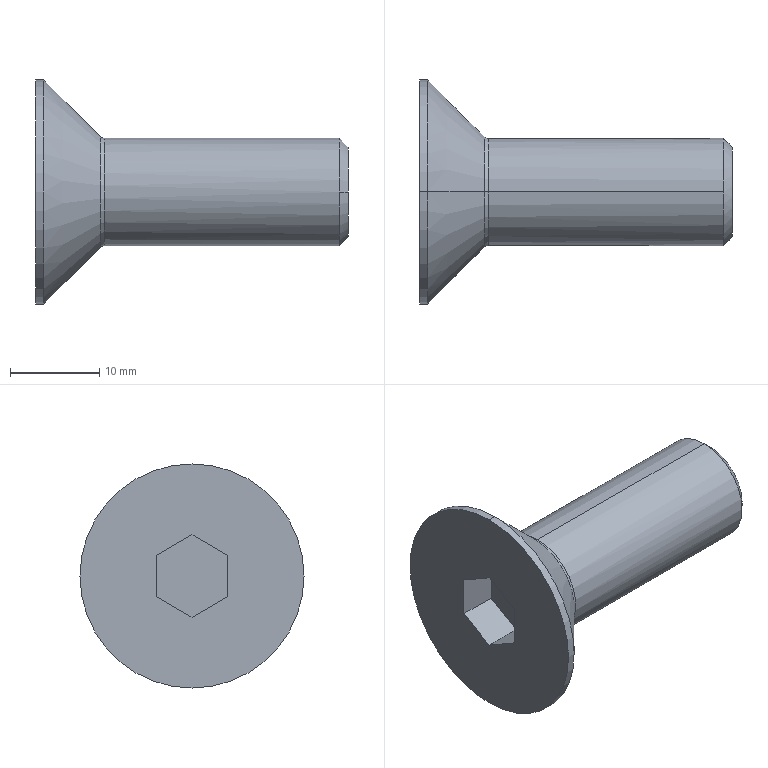Part | STEP file | 1 solid | 19 faces | box 35 x 25.075 x 25.075 mm | volume 5144 mm3 | plane 9 | cylinder 4 | cone 4 | spline 2 | commonest cylinder face diameters 12 x2 25.075 x2
STEP:
#1=CARTESIAN_POINT('',(0.,0.,0.));
#2=DIRECTION('',(0.,0.,1.));
#3=DIRECTION('',(1.,0.,0.));
#4=AXIS2_PLACEMENT_3D('',#1,#2,#3);
#5=CARTESIAN_POINT('',(-3.14,-4.,-2.309));
#6=VERTEX_POINT('',#5);
#7=CARTESIAN_POINT('',(-3.14,-4.,2.309));
#8=VERTEX_POINT('',#7);
#9=CARTESIAN_POINT('',(-3.14,-4.,-2.309));
#10=DIRECTION('',(0.,0.,1.));
#11=VECTOR('',#10,1.);
#12=LINE('',#9,#11);
#13=CARTESIAN_POINT('',(-3.14,0.,0.));
#14=DIRECTION('',(-1.,0.,0.));
#15=DIRECTION('',(0.,0.,1.));
#16=AXIS2_PLACEMENT_3D('',#13,#14,#15);
#17=PLANE('',#16);
#18=CARTESIAN_POINT('',(-2.309,-4.));
#19=DIRECTION('',(1.,0.));
#20=VECTOR('',#19,1.);
#21=LINE('',#18,#20);
#22=(GEOMETRIC_REPRESENTATION_CONTEXT(2)PARAMETRIC_REPRESENTATION_CONTEXT()REPRESENTATION_CONTEXT('',''));
#23=DEFINITIONAL_REPRESENTATION('',(#21),#22);
#24=PCURVE('',#17,#23);
#25=CARTESIAN_POINT('',(-3.14,-4.,-2.309));
#26=DIRECTION('',(0.,-1.,0.));
#27=DIRECTION('',(-1.,0.,0.));
#28=AXIS2_PLACEMENT_3D('',#25,#26,#27);
#29=PLANE('',#28);
#30=CARTESIAN_POINT('',(0.,0.));
#31=DIRECTION('',(0.,-1.));
#32=VECTOR('',#31,1.);
#33=LINE('',#30,#32);
#34=(GEOMETRIC_REPRESENTATION_CONTEXT(2)PARAMETRIC_REPRESENTATION_CONTEXT()REPRESENTATION_CONTEXT('',''));
#35=DEFINITIONAL_REPRESENTATION('',(#33),#34);
#36=PCURVE('',#29,#35);
#37=SURFACE_CURVE('',#12,(#24,#36),.PCURVE_S1.);
#38=EDGE_CURVE('',#6,#8,#37,.T.);
#39=ORIENTED_EDGE('',*,*,#38,.T.);
#40=CARTESIAN_POINT('',(-3.14,0.,4.619));
#41=VERTEX_POINT('',#40);
#42=CARTESIAN_POINT('',(-3.14,-4.,2.309));
#43=DIRECTION('',(0.,0.866,0.5));
#44=VECTOR('',#43,1.);
#45=LINE('',#42,#44);
#46=CARTESIAN_POINT('',(2.309,-4.));
#47=DIRECTION('',(0.5,0.866));
#48=VECTOR('',#47,1.);
#49=LINE('',#46,#48);
#50=(GEOMETRIC_REPRESENTATION_CONTEXT(2)PARAMETRIC_REPRESENTATION_CONTEXT()REPRESENTATION_CONTEXT('',''));
#51=DEFINITIONAL_REPRESENTATION('',(#49),#50);
#52=PCURVE('',#17,#51);
#53=CARTESIAN_POINT('',(-3.14,-4.,2.309));
#54=DIRECTION('',(0.,-0.5,0.866));
#55=DIRECTION('',(-1.,0.,0.));
#56=AXIS2_PLACEMENT_3D('',#53,#54,#55);
#57=PLANE('',#56);
#58=CARTESIAN_POINT('',(0.,0.));
#59=DIRECTION('',(0.,-1.));
#60=VECTOR('',#59,1.);
#61=LINE('',#58,#60);
#62=(GEOMETRIC_REPRESENTATION_CONTEXT(2)PARAMETRIC_REPRESENTATION_CONTEXT()REPRESENTATION_CONTEXT('',''));
#63=DEFINITIONAL_REPRESENTATION('',(#61),#62);
#64=PCURVE('',#57,#63);
#65=SURFACE_CURVE('',#45,(#52,#64),.PCURVE_S1.);
#66=EDGE_CURVE('',#8,#41,#65,.T.);
#67=ORIENTED_EDGE('',*,*,#66,.T.);
#68=CARTESIAN_POINT('',(-3.14,4.,2.309));
#69=VERTEX_POINT('',#68);
#70=CARTESIAN_POINT('',(-3.14,0.,4.619));
#71=DIRECTION('',(0.,0.866,-0.5));
#72=VECTOR('',#71,1.);
#73=LINE('',#70,#72);
#74=CARTESIAN_POINT('',(4.619,0.));
#75=DIRECTION('',(-0.5,0.866));
#76=VECTOR('',#75,1.);
#77=LINE('',#74,#76);
#78=(GEOMETRIC_REPRESENTATION_CONTEXT(2)PARAMETRIC_REPRESENTATION_CONTEXT()REPRESENTATION_CONTEXT('',''));
#79=DEFINITIONAL_REPRESENTATION('',(#77),#78);
#80=PCURVE('',#17,#79);
#81=CARTESIAN_POINT('',(-3.14,0.,4.619));
#82=DIRECTION('',(0.,0.5,0.866));
#83=DIRECTION('',(1.,0.,0.));
#84=AXIS2_PLACEMENT_3D('',#81,#82,#83);
#85=PLANE('',#84);
#86=CARTESIAN_POINT('',(0.,0.));
#87=DIRECTION('',(0.,1.));
#88=VECTOR('',#87,1.);
#89=LINE('',#86,#88);
#90=(GEOMETRIC_REPRESENTATION_CONTEXT(2)PARAMETRIC_REPRESENTATION_CONTEXT()REPRESENTATION_CONTEXT('',''));
#91=DEFINITIONAL_REPRESENTATION('',(#89),#90);
#92=PCURVE('',#85,#91);
#93=SURFACE_CURVE('',#73,(#80,#92),.PCURVE_S1.);
#94=EDGE_CURVE('',#41,#69,#93,.T.);
#95=ORIENTED_EDGE('',*,*,#94,.T.);
#96=CARTESIAN_POINT('',(-3.14,4.,-2.309));
#97=VERTEX_POINT('',#96);
#98=CARTESIAN_POINT('',(-3.14,4.,2.309));
#99=DIRECTION('',(0.,0.,-1.));
#100=VECTOR('',#99,1.);
#101=LINE('',#98,#100);
#102=CARTESIAN_POINT('',(2.309,4.));
#103=DIRECTION('',(-1.,0.));
#104=VECTOR('',#103,1.);
#105=LINE('',#102,#104);
#106=(GEOMETRIC_REPRESENTATION_CONTEXT(2)PARAMETRIC_REPRESENTATION_CONTEXT()REPRESENTATION_CONTEXT('',''));
#107=DEFINITIONAL_REPRESENTATION('',(#105),#106);
#108=PCURVE('',#17,#107);
#109=CARTESIAN_POINT('',(-3.14,4.,2.309));
#110=DIRECTION('',(0.,1.,0.));
#111=DIRECTION('',(1.,0.,0.));
#112=AXIS2_PLACEMENT_3D('',#109,#110,#111);
#113=PLANE('',#112);
#114=CARTESIAN_POINT('',(0.,0.));
#115=DIRECTION('',(0.,1.));
#116=VECTOR('',#115,1.);
#117=LINE('',#114,#116);
#118=(GEOMETRIC_REPRESENTATION_CONTEXT(2)PARAMETRIC_REPRESENTATION_CONTEXT()REPRESENTATION_CONTEXT('',''));
#119=DEFINITIONAL_REPRESENTATION('',(#117),#118);
#120=PCURVE('',#113,#119);
#121=SURFACE_CURVE('',#101,(#108,#120),.PCURVE_S1.);
#122=EDGE_CURVE('',#69,#97,#121,.T.);
#123=ORIENTED_EDGE('',*,*,#122,.T.);
#124=CARTESIAN_POINT('',(-3.14,0.,-4.619));
#125=VERTEX_POINT('',#124);
#126=CARTESIAN_POINT('',(-3.14,4.,-2.309));
#127=DIRECTION('',(0.,-0.866,-0.5));
#128=VECTOR('',#127,1.);
#129=LINE('',#126,#128);
#130=CARTESIAN_POINT('',(-2.309,4.));
#131=DIRECTION('',(-0.5,-0.866));
#132=VECTOR('',#131,1.);
#133=LINE('',#130,#132);
#134=(GEOMETRIC_REPRESENTATION_CONTEXT(2)PARAMETRIC_REPRESENTATION_CONTEXT()REPRESENTATION_CONTEXT('',''));
#135=DEFINITIONAL_REPRESENTATION('',(#133),#134);
#136=PCURVE('',#17,#135);
#137=CARTESIAN_POINT('',(-3.14,4.,-2.309));
#138=DIRECTION('',(0.,0.5,-0.866));
#139=DIRECTION('',(-1.,0.,0.));
#140=AXIS2_PLACEMENT_3D('',#137,#138,#139);
#141=PLANE('',#140);
#142=CARTESIAN_POINT('',(0.,0.));
#143=DIRECTION('',(0.,-1.));
#144=VECTOR('',#143,1.);
#145=LINE('',#142,#144);
#146=(GEOMETRIC_REPRESENTATION_CONTEXT(2)PARAMETRIC_REPRESENTATION_CONTEXT()REPRESENTATION_CONTEXT('',''));
#147=DEFINITIONAL_REPRESENTATION('',(#145),#146);
#148=PCURVE('',#141,#147);
#149=SURFACE_CURVE('',#129,(#136,#148),.PCURVE_S1.);
#150=EDGE_CURVE('',#97,#125,#149,.T.);
#151=ORIENTED_EDGE('',*,*,#150,.T.);
#152=CARTESIAN_POINT('',(-3.14,0.,-4.619));
#153=DIRECTION('',(0.,-0.866,0.5));
#154=VECTOR('',#153,1.);
#155=LINE('',#152,#154);
#156=CARTESIAN_POINT('',(-4.619,0.));
#157=DIRECTION('',(0.5,-0.866));
#158=VECTOR('',#157,1.);
#159=LINE('',#156,#158);
#160=(GEOMETRIC_REPRESENTATION_CONTEXT(2)PARAMETRIC_REPRESENTATION_CONTEXT()REPRESENTATION_CONTEXT('',''));
#161=DEFINITIONAL_REPRESENTATION('',(#159),#160);
#162=PCURVE('',#17,#161);
#163=CARTESIAN_POINT('',(-3.14,0.,-4.619));
#164=DIRECTION('',(0.,-0.5,-0.866));
#165=DIRECTION('',(0.,-0.866,0.5));
#166=AXIS2_PLACEMENT_3D('',#163,#164,#165);
#167=PLANE('',#166);
#168=CARTESIAN_POINT('',(0.,0.));
#169=DIRECTION('',(1.,0.));
#170=VECTOR('',#169,1.);
#171=LINE('',#168,#170);
#172=(GEOMETRIC_REPRESENTATION_CONTEXT(2)PARAMETRIC_REPRESENTATION_CONTEXT()REPRESENTATION_CONTEXT('',''));
#173=DEFINITIONAL_REPRESENTATION('',(#171),#172);
#174=PCURVE('',#167,#173);
#175=SURFACE_CURVE('',#155,(#162,#174),.PCURVE_S1.);
#176=EDGE_CURVE('',#125,#6,#175,.T.);
#177=ORIENTED_EDGE('',*,*,#176,.T.);
#178=EDGE_LOOP('',(#39,#67,#95,#123,#151,#177));
#179=FACE_BOUND('',#178,.T.);
#180=ADVANCED_FACE('',(#179),#17,.T.);
#181=CARTESIAN_POINT('',(-7.44,0.,-4.619));
#182=VERTEX_POINT('',#181);
#183=CARTESIAN_POINT('',(-3.14,0.,-4.619));
#184=DIRECTION('',(1.,0.,0.));
#185=VECTOR('',#184,1.);
#186=LINE('',#183,#185);
#187=CARTESIAN_POINT('',(0.,-4.619));
#188=DIRECTION('',(-1.,0.));
#189=VECTOR('',#188,1.);
#190=LINE('',#187,#189);
#191=(GEOMETRIC_REPRESENTATION_CONTEXT(2)PARAMETRIC_REPRESENTATION_CONTEXT()REPRESENTATION_CONTEXT('',''));
#192=DEFINITIONAL_REPRESENTATION('',(#190),#191);
#193=PCURVE('',#141,#192);
#194=CARTESIAN_POINT('',(0.,0.));
#195=DIRECTION('',(0.,-1.));
#196=VECTOR('',#195,1.);
#197=LINE('',#194,#196);
#198=(GEOMETRIC_REPRESENTATION_CONTEXT(2)PARAMETRIC_REPRESENTATION_CONTEXT()REPRESENTATION_CONTEXT('',''));
#199=DEFINITIONAL_REPRESENTATION('',(#197),#198);
#200=PCURVE('',#167,#199);
#201=SURFACE_CURVE('',#186,(#193,#200),.PCURVE_S1.);
#202=EDGE_CURVE('',#182,#125,#201,.T.);
#203=ORIENTED_EDGE('',*,*,#202,.T.);
#204=ORIENTED_EDGE('',*,*,#150,.F.);
#205=CARTESIAN_POINT('',(-7.44,4.,-2.309));
#206=VERTEX_POINT('',#205);
#207=CARTESIAN_POINT('',(-3.14,4.,-2.309));
#208=DIRECTION('',(-1.,0.,0.));
#209=VECTOR('',#208,1.);
#210=LINE('',#207,#209);
#211=CARTESIAN_POINT('',(0.,0.));
#212=DIRECTION('',(1.,0.));
#213=VECTOR('',#212,1.);
#214=LINE('',#211,#213);
#215=(GEOMETRIC_REPRESENTATION_CONTEXT(2)PARAMETRIC_REPRESENTATION_CONTEXT()REPRESENTATION_CONTEXT('',''));
#216=DEFINITIONAL_REPRESENTATION('',(#214),#215);
#217=PCURVE('',#141,#216);
#218=CARTESIAN_POINT('',(0.,4.619));
#219=DIRECTION('',(-1.,0.));
#220=VECTOR('',#219,1.);
#221=LINE('',#218,#220);
#222=(GEOMETRIC_REPRESENTATION_CONTEXT(2)PARAMETRIC_REPRESENTATION_CONTEXT()REPRESENTATION_CONTEXT('',''));
#223=DEFINITIONAL_REPRESENTATION('',(#221),#222);
#224=PCURVE('',#113,#223);
#225=SURFACE_CURVE('',#210,(#217,#224),.PCURVE_S1.);
#226=EDGE_CURVE('',#97,#206,#225,.T.);
#227=ORIENTED_EDGE('',*,*,#226,.T.);
#228=CARTESIAN_POINT('',(-7.44,4.,-2.309));
#229=DIRECTION('',(0.,-0.866,-0.5));
#230=VECTOR('',#229,1.);
#231=LINE('',#228,#230);
#232=CARTESIAN_POINT('',(4.3,0.));
#233=DIRECTION('',(0.,-1.));
#234=VECTOR('',#233,1.);
#235=LINE('',#232,#234);
#236=(GEOMETRIC_REPRESENTATION_CONTEXT(2)PARAMETRIC_REPRESENTATION_CONTEXT()REPRESENTATION_CONTEXT('',''));
#237=DEFINITIONAL_REPRESENTATION('',(#235),#236);
#238=PCURVE('',#141,#237);
#239=CARTESIAN_POINT('',(-7.44,12.537,0.));
#240=DIRECTION('',(1.,0.,0.));
#241=DIRECTION('',(0.,1.,0.));
#242=AXIS2_PLACEMENT_3D('',#239,#240,#241);
#243=PLANE('',#242);
#244=CARTESIAN_POINT('',(-8.537,-2.309));
#245=DIRECTION('',(-0.866,-0.5));
#246=VECTOR('',#245,1.);
#247=LINE('',#244,#246);
#248=(GEOMETRIC_REPRESENTATION_CONTEXT(2)PARAMETRIC_REPRESENTATION_CONTEXT()REPRESENTATION_CONTEXT('',''));
#249=DEFINITIONAL_REPRESENTATION('',(#247),#248);
#250=PCURVE('',#243,#249);
#251=SURFACE_CURVE('',#231,(#238,#250),.PCURVE_S1.);
#252=EDGE_CURVE('',#206,#182,#251,.T.);
#253=ORIENTED_EDGE('',*,*,#252,.T.);
#254=EDGE_LOOP('',(#203,#204,#227,#253));
#255=FACE_BOUND('',#254,.T.);
#256=ADVANCED_FACE('',(#255),#141,.F.);
#257=CARTESIAN_POINT('',(-7.44,-4.,-2.309));
#258=VERTEX_POINT('',#257);
#259=CARTESIAN_POINT('',(-3.14,-4.,-2.309));
#260=DIRECTION('',(1.,0.,0.));
#261=VECTOR('',#260,1.);
#262=LINE('',#259,#261);
#263=CARTESIAN_POINT('',(4.619,0.));
#264=DIRECTION('',(0.,-1.));
#265=VECTOR('',#264,1.);
#266=LINE('',#263,#265);
#267=(GEOMETRIC_REPRESENTATION_CONTEXT(2)PARAMETRIC_REPRESENTATION_CONTEXT()REPRESENTATION_CONTEXT('',''));
#268=DEFINITIONAL_REPRESENTATION('',(#266),#267);
#269=PCURVE('',#167,#268);
#270=CARTESIAN_POINT('',(0.,0.));
#271=DIRECTION('',(-1.,0.));
#272=VECTOR('',#271,1.);
#273=LINE('',#270,#272);
#274=(GEOMETRIC_REPRESENTATION_CONTEXT(2)PARAMETRIC_REPRESENTATION_CONTEXT()REPRESENTATION_CONTEXT('',''));
#275=DEFINITIONAL_REPRESENTATION('',(#273),#274);
#276=PCURVE('',#29,#275);
#277=SURFACE_CURVE('',#262,(#269,#276),.PCURVE_S1.);
#278=EDGE_CURVE('',#258,#6,#277,.T.);
#279=ORIENTED_EDGE('',*,*,#278,.T.);
#280=ORIENTED_EDGE('',*,*,#176,.F.);
#281=ORIENTED_EDGE('',*,*,#202,.F.);
#282=CARTESIAN_POINT('',(-7.44,0.,-4.619));
#283=DIRECTION('',(0.,-0.866,0.5));
#284=VECTOR('',#283,1.);
#285=LINE('',#282,#284);
#286=CARTESIAN_POINT('',(0.,4.3));
#287=DIRECTION('',(1.,0.));
#288=VECTOR('',#287,1.);
#289=LINE('',#286,#288);
#290=(GEOMETRIC_REPRESENTATION_CONTEXT(2)PARAMETRIC_REPRESENTATION_CONTEXT()REPRESENTATION_CONTEXT('',''));
#291=DEFINITIONAL_REPRESENTATION('',(#289),#290);
#292=PCURVE('',#167,#291);
#293=CARTESIAN_POINT('',(-12.537,-4.619));
#294=DIRECTION('',(-0.866,0.5));
#295=VECTOR('',#294,1.);
#296=LINE('',#293,#295);
#297=(GEOMETRIC_REPRESENTATION_CONTEXT(2)PARAMETRIC_REPRESENTATION_CONTEXT()REPRESENTATION_CONTEXT('',''));
#298=DEFINITIONAL_REPRESENTATION('',(#296),#297);
#299=PCURVE('',#243,#298);
#300=SURFACE_CURVE('',#285,(#292,#299),.PCURVE_S1.);
#301=EDGE_CURVE('',#182,#258,#300,.T.);
#302=ORIENTED_EDGE('',*,*,#301,.T.);
#303=EDGE_LOOP('',(#279,#280,#281,#302));
#304=FACE_BOUND('',#303,.T.);
#305=ADVANCED_FACE('',(#304),#167,.F.);
#306=CARTESIAN_POINT('',(-7.44,-4.,2.309));
#307=VERTEX_POINT('',#306);
#308=CARTESIAN_POINT('',(-3.14,-4.,2.309));
#309=DIRECTION('',(1.,0.,0.));
#310=VECTOR('',#309,1.);
#311=LINE('',#308,#310);
#312=CARTESIAN_POINT('',(0.,-4.619));
#313=DIRECTION('',(-1.,0.));
#314=VECTOR('',#313,1.);
#315=LINE('',#312,#314);
#316=(GEOMETRIC_REPRESENTATION_CONTEXT(2)PARAMETRIC_REPRESENTATION_CONTEXT()REPRESENTATION_CONTEXT('',''));
#317=DEFINITIONAL_REPRESENTATION('',(#315),#316);
#318=PCURVE('',#29,#317);
#319=CARTESIAN_POINT('',(0.,0.));
#320=DIRECTION('',(-1.,0.));
#321=VECTOR('',#320,1.);
#322=LINE('',#319,#321);
#323=(GEOMETRIC_REPRESENTATION_CONTEXT(2)PARAMETRIC_REPRESENTATION_CONTEXT()REPRESENTATION_CONTEXT('',''));
#324=DEFINITIONAL_REPRESENTATION('',(#322),#323);
#325=PCURVE('',#57,#324);
#326=SURFACE_CURVE('',#311,(#318,#325),.PCURVE_S1.);
#327=EDGE_CURVE('',#307,#8,#326,.T.);
#328=ORIENTED_EDGE('',*,*,#327,.T.);
#329=ORIENTED_EDGE('',*,*,#38,.F.);
#330=ORIENTED_EDGE('',*,*,#278,.F.);
#331=CARTESIAN_POINT('',(-7.44,-4.,0.));
#332=DIRECTION('',(0.,0.,1.));
#333=VECTOR('',#332,1.);
#334=LINE('',#331,#333);
#335=CARTESIAN_POINT('',(4.3,-2.309));
#336=DIRECTION('',(0.,-1.));
#337=VECTOR('',#336,1.);
#338=LINE('',#335,#337);
#339=(GEOMETRIC_REPRESENTATION_CONTEXT(2)PARAMETRIC_REPRESENTATION_CONTEXT()REPRESENTATION_CONTEXT('',''));
#340=DEFINITIONAL_REPRESENTATION('',(#338),#339);
#341=PCURVE('',#29,#340);
#342=CARTESIAN_POINT('',(-16.537,0.));
#343=DIRECTION('',(0.,1.));
#344=VECTOR('',#343,1.);
#345=LINE('',#342,#344);
#346=(GEOMETRIC_REPRESENTATION_CONTEXT(2)PARAMETRIC_REPRESENTATION_CONTEXT()REPRESENTATION_CONTEXT('',''));
#347=DEFINITIONAL_REPRESENTATION('',(#345),#346);
#348=PCURVE('',#243,#347);
#349=SURFACE_CURVE('',#334,(#341,#348),.PCURVE_S1.);
#350=EDGE_CURVE('',#258,#307,#349,.T.);
#351=ORIENTED_EDGE('',*,*,#350,.T.);
#352=EDGE_LOOP('',(#328,#329,#330,#351));
#353=FACE_BOUND('',#352,.T.);
#354=ADVANCED_FACE('',(#353),#29,.F.);
#355=CARTESIAN_POINT('',(-7.44,0.,4.619));
#356=VERTEX_POINT('',#355);
#357=CARTESIAN_POINT('',(-3.14,0.,4.619));
#358=DIRECTION('',(1.,0.,0.));
#359=VECTOR('',#358,1.);
#360=LINE('',#357,#359);
#361=CARTESIAN_POINT('',(0.,-4.619));
#362=DIRECTION('',(-1.,0.));
#363=VECTOR('',#362,1.);
#364=LINE('',#361,#363);
#365=(GEOMETRIC_REPRESENTATION_CONTEXT(2)PARAMETRIC_REPRESENTATION_CONTEXT()REPRESENTATION_CONTEXT('',''));
#366=DEFINITIONAL_REPRESENTATION('',(#364),#365);
#367=PCURVE('',#57,#366);
#368=CARTESIAN_POINT('',(0.,0.));
#369=DIRECTION('',(1.,0.));
#370=VECTOR('',#369,1.);
#371=LINE('',#368,#370);
#372=(GEOMETRIC_REPRESENTATION_CONTEXT(2)PARAMETRIC_REPRESENTATION_CONTEXT()REPRESENTATION_CONTEXT('',''));
#373=DEFINITIONAL_REPRESENTATION('',(#371),#372);
#374=PCURVE('',#85,#373);
#375=SURFACE_CURVE('',#360,(#367,#374),.PCURVE_S1.);
#376=EDGE_CURVE('',#356,#41,#375,.T.);
#377=ORIENTED_EDGE('',*,*,#376,.T.);
#378=ORIENTED_EDGE('',*,*,#66,.F.);
#379=ORIENTED_EDGE('',*,*,#327,.F.);
#380=CARTESIAN_POINT('',(-7.44,-4.,2.309));
#381=DIRECTION('',(0.,0.866,0.5));
#382=VECTOR('',#381,1.);
#383=LINE('',#380,#382);
#384=CARTESIAN_POINT('',(4.3,0.));
#385=DIRECTION('',(0.,-1.));
#386=VECTOR('',#385,1.);
#387=LINE('',#384,#386);
#388=(GEOMETRIC_REPRESENTATION_CONTEXT(2)PARAMETRIC_REPRESENTATION_CONTEXT()REPRESENTATION_CONTEXT('',''));
#389=DEFINITIONAL_REPRESENTATION('',(#387),#388);
#390=PCURVE('',#57,#389);
#391=CARTESIAN_POINT('',(-16.537,2.309));
#392=DIRECTION('',(0.866,0.5));
#393=VECTOR('',#392,1.);
#394=LINE('',#391,#393);
#395=(GEOMETRIC_REPRESENTATION_CONTEXT(2)PARAMETRIC_REPRESENTATION_CONTEXT()REPRESENTATION_CONTEXT('',''));
#396=DEFINITIONAL_REPRESENTATION('',(#394),#395);
#397=PCURVE('',#243,#396);
#398=SURFACE_CURVE('',#383,(#390,#397),.PCURVE_S1.);
#399=EDGE_CURVE('',#307,#356,#398,.T.);
#400=ORIENTED_EDGE('',*,*,#399,.T.);
#401=EDGE_LOOP('',(#377,#378,#379,#400));
#402=FACE_BOUND('',#401,.T.);
#403=ADVANCED_FACE('',(#402),#57,.F.);
#404=CARTESIAN_POINT('',(-7.44,4.,2.309));
#405=VERTEX_POINT('',#404);
#406=CARTESIAN_POINT('',(-3.14,4.,2.309));
#407=DIRECTION('',(1.,0.,0.));
#408=VECTOR('',#407,1.);
#409=LINE('',#406,#408);
#410=CARTESIAN_POINT('',(0.,4.619));
#411=DIRECTION('',(1.,0.));
#412=VECTOR('',#411,1.);
#413=LINE('',#410,#412);
#414=(GEOMETRIC_REPRESENTATION_CONTEXT(2)PARAMETRIC_REPRESENTATION_CONTEXT()REPRESENTATION_CONTEXT('',''));
#415=DEFINITIONAL_REPRESENTATION('',(#413),#414);
#416=PCURVE('',#85,#415);
#417=CARTESIAN_POINT('',(0.,0.));
#418=DIRECTION('',(1.,0.));
#419=VECTOR('',#418,1.);
#420=LINE('',#417,#419);
#421=(GEOMETRIC_REPRESENTATION_CONTEXT(2)PARAMETRIC_REPRESENTATION_CONTEXT()REPRESENTATION_CONTEXT('',''));
#422=DEFINITIONAL_REPRESENTATION('',(#420),#421);
#423=PCURVE('',#113,#422);
#424=SURFACE_CURVE('',#409,(#416,#423),.PCURVE_S1.);
#425=EDGE_CURVE('',#405,#69,#424,.T.);
#426=ORIENTED_EDGE('',*,*,#425,.T.);
#427=ORIENTED_EDGE('',*,*,#94,.F.);
#428=ORIENTED_EDGE('',*,*,#376,.F.);
#429=CARTESIAN_POINT('',(-7.44,0.,4.619));
#430=DIRECTION('',(0.,0.866,-0.5));
#431=VECTOR('',#430,1.);
#432=LINE('',#429,#431);
#433=CARTESIAN_POINT('',(-4.3,0.));
#434=DIRECTION('',(0.,1.));
#435=VECTOR('',#434,1.);
#436=LINE('',#433,#435);
#437=(GEOMETRIC_REPRESENTATION_CONTEXT(2)PARAMETRIC_REPRESENTATION_CONTEXT()REPRESENTATION_CONTEXT('',''));
#438=DEFINITIONAL_REPRESENTATION('',(#436),#437);
#439=PCURVE('',#85,#438);
#440=CARTESIAN_POINT('',(-12.537,4.619));
#441=DIRECTION('',(0.866,-0.5));
#442=VECTOR('',#441,1.);
#443=LINE('',#440,#442);
#444=(GEOMETRIC_REPRESENTATION_CONTEXT(2)PARAMETRIC_REPRESENTATION_CONTEXT()REPRESENTATION_CONTEXT('',''));
#445=DEFINITIONAL_REPRESENTATION('',(#443),#444);
#446=PCURVE('',#243,#445);
#447=SURFACE_CURVE('',#432,(#439,#446),.PCURVE_S1.);
#448=EDGE_CURVE('',#356,#405,#447,.T.);
#449=ORIENTED_EDGE('',*,*,#448,.T.);
#450=EDGE_LOOP('',(#426,#427,#428,#449));
#451=FACE_BOUND('',#450,.T.);
#452=ADVANCED_FACE('',(#451),#85,.F.);
#453=ORIENTED_EDGE('',*,*,#226,.F.);
#454=ORIENTED_EDGE('',*,*,#122,.F.);
#455=ORIENTED_EDGE('',*,*,#425,.F.);
#456=CARTESIAN_POINT('',(-7.44,4.,0.));
#457=DIRECTION('',(0.,0.,-1.));
#458=VECTOR('',#457,1.);
#459=LINE('',#456,#458);
#460=CARTESIAN_POINT('',(-4.3,2.309));
#461=DIRECTION('',(0.,1.));
#462=VECTOR('',#461,1.);
#463=LINE('',#460,#462);
#464=(GEOMETRIC_REPRESENTATION_CONTEXT(2)PARAMETRIC_REPRESENTATION_CONTEXT()REPRESENTATION_CONTEXT('',''));
#465=DEFINITIONAL_REPRESENTATION('',(#463),#464);
#466=PCURVE('',#113,#465);
#467=CARTESIAN_POINT('',(-8.537,0.));
#468=DIRECTION('',(0.,-1.));
#469=VECTOR('',#468,1.);
#470=LINE('',#467,#469);
#471=(GEOMETRIC_REPRESENTATION_CONTEXT(2)PARAMETRIC_REPRESENTATION_CONTEXT()REPRESENTATION_CONTEXT('',''));
#472=DEFINITIONAL_REPRESENTATION('',(#470),#471);
#473=PCURVE('',#243,#472);
#474=SURFACE_CURVE('',#459,(#466,#473),.PCURVE_S1.);
#475=EDGE_CURVE('',#405,#206,#474,.T.);
#476=ORIENTED_EDGE('',*,*,#475,.T.);
#477=EDGE_LOOP('',(#453,#454,#455,#476));
#478=FACE_BOUND('',#477,.T.);
#479=ADVANCED_FACE('',(#478),#113,.F.);
#480=ORIENTED_EDGE('',*,*,#448,.F.);
#481=ORIENTED_EDGE('',*,*,#399,.F.);
#482=ORIENTED_EDGE('',*,*,#350,.F.);
#483=ORIENTED_EDGE('',*,*,#301,.F.);
#484=ORIENTED_EDGE('',*,*,#252,.F.);
#485=ORIENTED_EDGE('',*,*,#475,.F.);
#486=EDGE_LOOP('',(#480,#481,#482,#483,#484,#485));
#487=FACE_BOUND('',#486,.T.);
#488=CARTESIAN_POINT('',(-7.44,0.,12.537));
#489=VERTEX_POINT('',#488);
#490=CARTESIAN_POINT('',(-7.44,0.,-12.537));
#491=VERTEX_POINT('',#490);
#492=CARTESIAN_POINT('',(-7.44,0.,0.));
#493=DIRECTION('',(1.,0.,0.));
#494=DIRECTION('',(0.,0.,1.));
#495=AXIS2_PLACEMENT_3D('',#492,#493,#494);
#496=CIRCLE('',#495,12.537);
#497=CARTESIAN_POINT('',(-12.537,0.));
#498=DIRECTION('',(0.,1.));
#499=AXIS2_PLACEMENT_2D('',#497,#498);
#500=CIRCLE('',#499,12.537);
#501=(GEOMETRIC_REPRESENTATION_CONTEXT(2)PARAMETRIC_REPRESENTATION_CONTEXT()REPRESENTATION_CONTEXT('',''));
#502=DEFINITIONAL_REPRESENTATION('',(#500),#501);
#503=PCURVE('',#243,#502);
#504=CARTESIAN_POINT('',(-37.991,0.,0.));
#505=DIRECTION('',(-1.,0.,0.));
#506=DIRECTION('',(0.,0.,1.));
#507=AXIS2_PLACEMENT_3D('',#504,#505,#506);
#508=CYLINDRICAL_SURFACE('',#507,12.537);
#509=CARTESIAN_POINT('',(6.283,-30.551));
#510=DIRECTION('',(-1.,0.));
#511=VECTOR('',#510,1.);
#512=LINE('',#509,#511);
#513=(GEOMETRIC_REPRESENTATION_CONTEXT(2)PARAMETRIC_REPRESENTATION_CONTEXT()REPRESENTATION_CONTEXT('',''));
#514=DEFINITIONAL_REPRESENTATION('',(#512),#513);
#515=PCURVE('',#508,#514);
#516=SURFACE_CURVE('',#496,(#503,#515),.PCURVE_S1.);
#517=EDGE_CURVE('',#489,#491,#516,.T.);
#518=ORIENTED_EDGE('',*,*,#517,.F.);
#519=CARTESIAN_POINT('',(-7.44,0.,0.));
#520=DIRECTION('',(1.,0.,0.));
#521=DIRECTION('',(0.,0.,1.));
#522=AXIS2_PLACEMENT_3D('',#519,#520,#521);
#523=CIRCLE('',#522,12.537);
#524=CARTESIAN_POINT('',(-12.537,0.));
#525=DIRECTION('',(0.,1.));
#526=AXIS2_PLACEMENT_2D('',#524,#525);
#527=CIRCLE('',#526,12.537);
#528=(GEOMETRIC_REPRESENTATION_CONTEXT(2)PARAMETRIC_REPRESENTATION_CONTEXT()REPRESENTATION_CONTEXT('',''));
#529=DEFINITIONAL_REPRESENTATION('',(#527),#528);
#530=PCURVE('',#243,#529);
#531=CARTESIAN_POINT('',(-37.991,0.,0.));
#532=DIRECTION('',(-1.,0.,0.));
#533=DIRECTION('',(0.,0.,1.));
#534=AXIS2_PLACEMENT_3D('',#531,#532,#533);
#535=CYLINDRICAL_SURFACE('',#534,12.537);
#536=CARTESIAN_POINT('',(6.283,-30.551));
#537=DIRECTION('',(-1.,0.));
#538=VECTOR('',#537,1.);
#539=LINE('',#536,#538);
#540=(GEOMETRIC_REPRESENTATION_CONTEXT(2)PARAMETRIC_REPRESENTATION_CONTEXT()REPRESENTATION_CONTEXT('',''));
#541=DEFINITIONAL_REPRESENTATION('',(#539),#540);
#542=PCURVE('',#535,#541);
#543=SURFACE_CURVE('',#523,(#530,#542),.PCURVE_S1.);
#544=EDGE_CURVE('',#491,#489,#543,.T.);
#545=ORIENTED_EDGE('',*,*,#544,.F.);
#546=EDGE_LOOP('',(#518,#545));
#547=FACE_BOUND('',#546,.T.);
#548=ADVANCED_FACE('',(#487,#547),#243,.F.);
#549=CARTESIAN_POINT('',(-6.537,0.,-12.537));
#550=VERTEX_POINT('',#549);
#551=CARTESIAN_POINT('',(-37.991,0.,-12.537));
#552=DIRECTION('',(-1.,0.,0.));
#553=VECTOR('',#552,1.);
#554=LINE('',#551,#553);
#555=CARTESIAN_POINT('',(3.142,0.));
#556=DIRECTION('',(0.,1.));
#557=VECTOR('',#556,1.);
#558=LINE('',#555,#557);
#559=(GEOMETRIC_REPRESENTATION_CONTEXT(2)PARAMETRIC_REPRESENTATION_CONTEXT()REPRESENTATION_CONTEXT('',''));
#560=DEFINITIONAL_REPRESENTATION('',(#558),#559);
#561=PCURVE('',#508,#560);
#562=CARTESIAN_POINT('',(3.142,0.));
#563=DIRECTION('',(0.,1.));
#564=VECTOR('',#563,1.);
#565=LINE('',#562,#564);
#566=(GEOMETRIC_REPRESENTATION_CONTEXT(2)PARAMETRIC_REPRESENTATION_CONTEXT()REPRESENTATION_CONTEXT('',''));
#567=DEFINITIONAL_REPRESENTATION('',(#565),#566);
#568=PCURVE('',#535,#567);
#569=SURFACE_CURVE('',#554,(#561,#568),.PCURVE_S1.);
#570=EDGE_CURVE('',#550,#491,#569,.T.);
#571=ORIENTED_EDGE('',*,*,#570,.F.);
#572=CARTESIAN_POINT('',(-6.537,0.,12.537));
#573=VERTEX_POINT('',#572);
#574=CARTESIAN_POINT('',(-6.537,0.,0.));
#575=DIRECTION('',(1.,0.,0.));
#576=DIRECTION('',(0.,0.,1.));
#577=AXIS2_PLACEMENT_3D('',#574,#575,#576);
#578=CIRCLE('',#577,12.537);
#579=CARTESIAN_POINT('',(6.283,-31.454));
#580=DIRECTION('',(-1.,0.));
#581=VECTOR('',#580,1.);
#582=LINE('',#579,#581);
#583=(GEOMETRIC_REPRESENTATION_CONTEXT(2)PARAMETRIC_REPRESENTATION_CONTEXT()REPRESENTATION_CONTEXT('',''));
#584=DEFINITIONAL_REPRESENTATION('',(#582),#583);
#585=PCURVE('',#508,#584);
#586=CARTESIAN_POINT('',(-6.537,0.,0.));
#587=DIRECTION('',(-1.,0.,0.));
#588=DIRECTION('',(0.,0.,1.));
#589=AXIS2_PLACEMENT_3D('',#586,#587,#588);
#590=CONICAL_SURFACE('',#589,12.537,0.7854);
#591=CARTESIAN_POINT('',(6.283,0.));
#592=DIRECTION('',(-1.,0.));
#593=VECTOR('',#592,1.);
#594=LINE('',#591,#593);
#595=(GEOMETRIC_REPRESENTATION_CONTEXT(2)PARAMETRIC_REPRESENTATION_CONTEXT()REPRESENTATION_CONTEXT('',''));
#596=DEFINITIONAL_REPRESENTATION('',(#594),#595);
#597=PCURVE('',#590,#596);
#598=SURFACE_CURVE('',#578,(#585,#597),.PCURVE_S1.);
#599=EDGE_CURVE('',#573,#550,#598,.T.);
#600=ORIENTED_EDGE('',*,*,#599,.F.);
#601=CARTESIAN_POINT('',(-37.991,0.,12.537));
#602=DIRECTION('',(-1.,0.,0.));
#603=VECTOR('',#602,1.);
#604=LINE('',#601,#603);
#605=CARTESIAN_POINT('',(6.283,0.));
#606=DIRECTION('',(0.,1.));
#607=VECTOR('',#606,1.);
#608=LINE('',#605,#607);
#609=(GEOMETRIC_REPRESENTATION_CONTEXT(2)PARAMETRIC_REPRESENTATION_CONTEXT()REPRESENTATION_CONTEXT('',''));
#610=DEFINITIONAL_REPRESENTATION('',(#608),#609);
#611=PCURVE('',#508,#610);
#612=CARTESIAN_POINT('',(0.,0.));
#613=DIRECTION('',(0.,1.));
#614=VECTOR('',#613,1.);
#615=LINE('',#612,#614);
#616=(GEOMETRIC_REPRESENTATION_CONTEXT(2)PARAMETRIC_REPRESENTATION_CONTEXT()REPRESENTATION_CONTEXT('',''));
#617=DEFINITIONAL_REPRESENTATION('',(#615),#616);
#618=PCURVE('',#535,#617);
#619=SURFACE_CURVE('',#604,(#611,#618),.PCURVE_S1.);
#620=EDGE_CURVE('',#573,#489,#619,.T.);
#621=ORIENTED_EDGE('',*,*,#620,.T.);
#622=ORIENTED_EDGE('',*,*,#517,.T.);
#623=EDGE_LOOP('',(#571,#600,#621,#622));
#624=FACE_BOUND('',#623,.T.);
#625=ADVANCED_FACE('',(#624),#508,.T.);
#626=CARTESIAN_POINT('',(27.56,-5.,0.));
#627=VERTEX_POINT('',#626);
#628=CARTESIAN_POINT('',(27.56,5.,0.));
#629=VERTEX_POINT('',#628);
#630=CARTESIAN_POINT('',(27.56,0.,0.));
#631=DIRECTION('',(-1.,0.,0.));
#632=DIRECTION('',(0.,-1.,0.));
#633=AXIS2_PLACEMENT_3D('',#630,#631,#632);
#634=CIRCLE('',#633,5.);
#635=CARTESIAN_POINT('',(27.56,6.,0.));
#636=DIRECTION('',(-1.,0.,0.));
#637=DIRECTION('',(0.,0.,1.));
#638=AXIS2_PLACEMENT_3D('',#635,#636,#637);
#639=PLANE('',#638);
#640=CARTESIAN_POINT('',(0.,-6.));
#641=DIRECTION('',(0.,-1.));
#642=AXIS2_PLACEMENT_2D('',#640,#641);
#643=CIRCLE('',#642,5.);
#644=(GEOMETRIC_REPRESENTATION_CONTEXT(2)PARAMETRIC_REPRESENTATION_CONTEXT()REPRESENTATION_CONTEXT('',''));
#645=DEFINITIONAL_REPRESENTATION('',(#643),#644);
#646=PCURVE('',#639,#645);
#647=CARTESIAN_POINT('',(26.56,0.,0.));
#648=DIRECTION('',(-1.,0.,0.));
#649=DIRECTION('',(0.,-1.,0.));
#650=AXIS2_PLACEMENT_3D('',#647,#648,#649);
#651=CONICAL_SURFACE('',#650,6.,0.7854);
#652=CARTESIAN_POINT('',(0.,-1.));
#653=DIRECTION('',(1.,0.));
#654=VECTOR('',#653,1.);
#655=LINE('',#652,#654);
#656=(GEOMETRIC_REPRESENTATION_CONTEXT(2)PARAMETRIC_REPRESENTATION_CONTEXT()REPRESENTATION_CONTEXT('',''));
#657=DEFINITIONAL_REPRESENTATION('',(#655),#656);
#658=PCURVE('',#651,#657);
#659=SURFACE_CURVE('',#634,(#646,#658),.PCURVE_S1.);
#660=EDGE_CURVE('',#627,#629,#659,.T.);
#661=ORIENTED_EDGE('',*,*,#660,.F.);
#662=CARTESIAN_POINT('',(27.56,0.,0.));
#663=DIRECTION('',(-1.,0.,0.));
#664=DIRECTION('',(0.,-1.,0.));
#665=AXIS2_PLACEMENT_3D('',#662,#663,#664);
#666=CIRCLE('',#665,5.);
#667=CARTESIAN_POINT('',(0.,-6.));
#668=DIRECTION('',(0.,-1.));
#669=AXIS2_PLACEMENT_2D('',#667,#668);
#670=CIRCLE('',#669,5.);
#671=(GEOMETRIC_REPRESENTATION_CONTEXT(2)PARAMETRIC_REPRESENTATION_CONTEXT()REPRESENTATION_CONTEXT('',''));
#672=DEFINITIONAL_REPRESENTATION('',(#670),#671);
#673=PCURVE('',#639,#672);
#674=CARTESIAN_POINT('',(26.56,0.,0.));
#675=DIRECTION('',(-1.,0.,0.));
#676=DIRECTION('',(0.,-1.,0.));
#677=AXIS2_PLACEMENT_3D('',#674,#675,#676);
#678=CONICAL_SURFACE('',#677,6.,0.7854);
#679=CARTESIAN_POINT('',(0.,-1.));
#680=DIRECTION('',(1.,0.));
#681=VECTOR('',#680,1.);
#682=LINE('',#679,#681);
#683=(GEOMETRIC_REPRESENTATION_CONTEXT(2)PARAMETRIC_REPRESENTATION_CONTEXT()REPRESENTATION_CONTEXT('',''));
#684=DEFINITIONAL_REPRESENTATION('',(#682),#683);
#685=PCURVE('',#678,#684);
#686=SURFACE_CURVE('',#666,(#673,#685),.PCURVE_S1.);
#687=EDGE_CURVE('',#629,#627,#686,.T.);
#688=ORIENTED_EDGE('',*,*,#687,.F.);
#689=EDGE_LOOP('',(#661,#688));
#690=FACE_BOUND('',#689,.T.);
#691=ADVANCED_FACE('',(#690),#639,.F.);
#692=CARTESIAN_POINT('',(-0.1757,0.,-6.176));
#693=VERTEX_POINT('',#692);
#694=CARTESIAN_POINT('',(-6.537,0.,-12.537));
#695=DIRECTION('',(-0.7071,0.,-0.7071));
#696=VECTOR('',#695,1.);
#697=LINE('',#694,#696);
#698=CARTESIAN_POINT('',(3.142,0.));
#699=DIRECTION('',(0.,1.));
#700=VECTOR('',#699,1.);
#701=LINE('',#698,#700);
#702=(GEOMETRIC_REPRESENTATION_CONTEXT(2)PARAMETRIC_REPRESENTATION_CONTEXT()REPRESENTATION_CONTEXT('',''));
#703=DEFINITIONAL_REPRESENTATION('',(#701),#702);
#704=PCURVE('',#590,#703);
#705=CARTESIAN_POINT('',(-6.537,0.,0.));
#706=DIRECTION('',(-1.,0.,0.));
#707=DIRECTION('',(0.,0.,1.));
#708=AXIS2_PLACEMENT_3D('',#705,#706,#707);
#709=CONICAL_SURFACE('',#708,12.537,0.7854);
#710=CARTESIAN_POINT('',(3.142,0.));
#711=DIRECTION('',(0.,1.));
#712=VECTOR('',#711,1.);
#713=LINE('',#710,#712);
#714=(GEOMETRIC_REPRESENTATION_CONTEXT(2)PARAMETRIC_REPRESENTATION_CONTEXT()REPRESENTATION_CONTEXT('',''));
#715=DEFINITIONAL_REPRESENTATION('',(#713),#714);
#716=PCURVE('',#709,#715);
#717=SURFACE_CURVE('',#697,(#704,#716),.PCURVE_S1.);
#718=EDGE_CURVE('',#693,#550,#717,.T.);
#719=ORIENTED_EDGE('',*,*,#718,.F.);
#720=CARTESIAN_POINT('',(-0.1757,0.,6.176));
#721=VERTEX_POINT('',#720);
#722=CARTESIAN_POINT('',(-0.1757,0.,0.));
#723=DIRECTION('',(-1.,0.,0.));
#724=DIRECTION('',(0.,0.,1.));
#725=AXIS2_PLACEMENT_3D('',#722,#723,#724);
#726=CIRCLE('',#725,6.176);
#727=CARTESIAN_POINT('',(0.,-6.362));
#728=DIRECTION('',(1.,0.));
#729=VECTOR('',#728,1.);
#730=LINE('',#727,#729);
#731=(GEOMETRIC_REPRESENTATION_CONTEXT(2)PARAMETRIC_REPRESENTATION_CONTEXT()REPRESENTATION_CONTEXT('',''));
#732=DEFINITIONAL_REPRESENTATION('',(#730),#731);
#733=PCURVE('',#590,#732);
#734=CARTESIAN_POINT('',(0.2485,0.,-6.));
#735=CARTESIAN_POINT('',(0.2485,-12.,-6.));
#736=CARTESIAN_POINT('',(0.2485,-12.,6.));
#737=CARTESIAN_POINT('',(0.2485,0.,6.));
#738=CARTESIAN_POINT('',(0.08727,0.,-6.));
#739=CARTESIAN_POINT('',(0.08727,-12.,-6.));
#740=CARTESIAN_POINT('',(0.08727,-12.,6.));
#741=CARTESIAN_POINT('',(0.08727,0.,6.));
#742=CARTESIAN_POINT('',(-0.06171,0.,-6.062));
#743=CARTESIAN_POINT('',(-0.06171,-12.123,-6.062));
#744=CARTESIAN_POINT('',(-0.06171,-12.123,6.062));
#745=CARTESIAN_POINT('',(-0.06171,0.,6.062));
#746=CARTESIAN_POINT('',(-0.1757,0.,-6.176));
#747=CARTESIAN_POINT('',(-0.1757,-12.351,-6.176));
#748=CARTESIAN_POINT('',(-0.1757,-12.351,6.176));
#749=CARTESIAN_POINT('',(-0.1757,0.,6.176));
#750=(BOUNDED_SURFACE()B_SPLINE_SURFACE(3,3,((#734,#735,#736,#737),(#738,#739,#740,#741),(#742,#743,#744,#745),(#746,#747,#748,#749)),.UNSPECIFIED.,.F.,.F.,.F.)B_SPLINE_SURFACE_WITH_KNOTS((4,4),(4,4),(0.,1.),(0.,1.),.PIECEWISE_BEZIER_KNOTS.)GEOMETRIC_REPRESENTATION_ITEM()RATIONAL_B_SPLINE_SURFACE(((1.,0.3333,0.3333,1.),(0.9493,0.3164,0.3164,0.9493),(0.9493,0.3164,0.3164,0.9493),(1.,0.3333,0.3333,1.)))REPRESENTATION_ITEM('')SURFACE());
#751=CARTESIAN_POINT('',(1.,0.));
#752=CARTESIAN_POINT('',(1.,0.02375));
#753=CARTESIAN_POINT('',(1.,0.06805));
#754=CARTESIAN_POINT('',(1.,0.1267));
#755=CARTESIAN_POINT('',(1.,0.1794));
#756=CARTESIAN_POINT('',(1.,0.2276));
#757=CARTESIAN_POINT('',(1.,0.2721));
#758=CARTESIAN_POINT('',(1.,0.3139));
#759=CARTESIAN_POINT('',(1.,0.3535));
#760=CARTESIAN_POINT('',(1.,0.3914));
#761=CARTESIAN_POINT('',(1.,0.4282));
#762=CARTESIAN_POINT('',(1.,0.4643));
#763=CARTESIAN_POINT('',(1.,0.5));
#764=CARTESIAN_POINT('',(1.,0.5357));
#765=CARTESIAN_POINT('',(1.,0.5718));
#766=CARTESIAN_POINT('',(1.,0.6086));
#767=CARTESIAN_POINT('',(1.,0.6465));
#768=CARTESIAN_POINT('',(1.,0.6861));
#769=CARTESIAN_POINT('',(1.,0.7279));
#770=CARTESIAN_POINT('',(1.,0.7724));
#771=CARTESIAN_POINT('',(1.,0.8206));
#772=CARTESIAN_POINT('',(1.,0.8733));
#773=CARTESIAN_POINT('',(1.,0.9319));
#774=CARTESIAN_POINT('',(1.,0.9763));
#775=CARTESIAN_POINT('',(1.,1.));
#776=B_SPLINE_CURVE_WITH_KNOTS('',3,(#751,#752,#753,#754,#755,#756,#757,#758,#759,#760,#761,#762,#763,#764,#765,#766,#767,#768,#769,#770,#771,#772,#773,#774,#775),.UNSPECIFIED.,.F.,.F.,(4,1,1,1,1,1,1,1,1,1,1,1,1,1,1,1,1,1,1,1,1,1,4),(3.142,3.284,3.427,3.57,3.713,3.856,3.998,4.141,4.284,4.427,4.57,4.712,4.855,4.998,5.141,5.284,5.426,5.569,5.712,5.855,5.998,6.14,6.283),.QUASI_UNIFORM_KNOTS.);
#777=(GEOMETRIC_REPRESENTATION_CONTEXT(2)PARAMETRIC_REPRESENTATION_CONTEXT()REPRESENTATION_CONTEXT('',''));
#778=DEFINITIONAL_REPRESENTATION('',(#776),#777);
#779=PCURVE('',#750,#778);
#780=SURFACE_CURVE('',#726,(#733,#779),.PCURVE_S1.);
#781=EDGE_CURVE('',#693,#721,#780,.T.);
#782=ORIENTED_EDGE('',*,*,#781,.T.);
#783=CARTESIAN_POINT('',(-6.537,0.,12.537));
#784=DIRECTION('',(-0.7071,0.,0.7071));
#785=VECTOR('',#784,1.);
#786=LINE('',#783,#785);
#787=CARTESIAN_POINT('',(6.283,0.));
#788=DIRECTION('',(0.,1.));
#789=VECTOR('',#788,1.);
#790=LINE('',#787,#789);
#791=(GEOMETRIC_REPRESENTATION_CONTEXT(2)PARAMETRIC_REPRESENTATION_CONTEXT()REPRESENTATION_CONTEXT('',''));
#792=DEFINITIONAL_REPRESENTATION('',(#790),#791);
#793=PCURVE('',#590,#792);
#794=CARTESIAN_POINT('',(0.,0.));
#795=DIRECTION('',(0.,1.));
#796=VECTOR('',#795,1.);
#797=LINE('',#794,#796);
#798=(GEOMETRIC_REPRESENTATION_CONTEXT(2)PARAMETRIC_REPRESENTATION_CONTEXT()REPRESENTATION_CONTEXT('',''));
#799=DEFINITIONAL_REPRESENTATION('',(#797),#798);
#800=PCURVE('',#709,#799);
#801=SURFACE_CURVE('',#786,(#793,#800),.PCURVE_S1.);
#802=EDGE_CURVE('',#721,#573,#801,.T.);
#803=ORIENTED_EDGE('',*,*,#802,.T.);
#804=ORIENTED_EDGE('',*,*,#599,.T.);
#805=EDGE_LOOP('',(#719,#782,#803,#804));
#806=FACE_BOUND('',#805,.T.);
#807=ADVANCED_FACE('',(#806),#590,.T.);
#808=CARTESIAN_POINT('',(26.56,6.,0.));
#809=VERTEX_POINT('',#808);
#810=CARTESIAN_POINT('',(26.56,6.,0.));
#811=DIRECTION('',(-0.7071,0.7071,0.));
#812=VECTOR('',#811,1.);
#813=LINE('',#810,#812);
#814=CARTESIAN_POINT('',(3.142,0.));
#815=DIRECTION('',(0.,1.));
#816=VECTOR('',#815,1.);
#817=LINE('',#814,#816);
#818=(GEOMETRIC_REPRESENTATION_CONTEXT(2)PARAMETRIC_REPRESENTATION_CONTEXT()REPRESENTATION_CONTEXT('',''));
#819=DEFINITIONAL_REPRESENTATION('',(#817),#818);
#820=PCURVE('',#678,#819);
#821=CARTESIAN_POINT('',(3.142,0.));
#822=DIRECTION('',(0.,1.));
#823=VECTOR('',#822,1.);
#824=LINE('',#821,#823);
#825=(GEOMETRIC_REPRESENTATION_CONTEXT(2)PARAMETRIC_REPRESENTATION_CONTEXT()REPRESENTATION_CONTEXT('',''));
#826=DEFINITIONAL_REPRESENTATION('',(#824),#825);
#827=PCURVE('',#651,#826);
#828=SURFACE_CURVE('',#813,(#820,#827),.PCURVE_S1.);
#829=EDGE_CURVE('',#629,#809,#828,.T.);
#830=ORIENTED_EDGE('',*,*,#829,.F.);
#831=ORIENTED_EDGE('',*,*,#687,.T.);
#832=CARTESIAN_POINT('',(26.56,-6.,0.));
#833=VERTEX_POINT('',#832);
#834=CARTESIAN_POINT('',(26.56,-6.,0.));
#835=DIRECTION('',(-0.7071,-0.7071,0.));
#836=VECTOR('',#835,1.);
#837=LINE('',#834,#836);
#838=CARTESIAN_POINT('',(6.283,0.));
#839=DIRECTION('',(0.,1.));
#840=VECTOR('',#839,1.);
#841=LINE('',#838,#840);
#842=(GEOMETRIC_REPRESENTATION_CONTEXT(2)PARAMETRIC_REPRESENTATION_CONTEXT()REPRESENTATION_CONTEXT('',''));
#843=DEFINITIONAL_REPRESENTATION('',(#841),#842);
#844=PCURVE('',#678,#843);
#845=CARTESIAN_POINT('',(0.,0.));
#846=DIRECTION('',(0.,1.));
#847=VECTOR('',#846,1.);
#848=LINE('',#845,#847);
#849=(GEOMETRIC_REPRESENTATION_CONTEXT(2)PARAMETRIC_REPRESENTATION_CONTEXT()REPRESENTATION_CONTEXT('',''));
#850=DEFINITIONAL_REPRESENTATION('',(#848),#849);
#851=PCURVE('',#651,#850);
#852=SURFACE_CURVE('',#837,(#844,#851),.PCURVE_S1.);
#853=EDGE_CURVE('',#627,#833,#852,.T.);
#854=ORIENTED_EDGE('',*,*,#853,.T.);
#855=CARTESIAN_POINT('',(26.56,0.,-6.));
#856=VERTEX_POINT('',#855);
#857=CARTESIAN_POINT('',(26.56,0.,0.));
#858=DIRECTION('',(-1.,0.,0.));
#859=DIRECTION('',(0.,0.,1.));
#860=AXIS2_PLACEMENT_3D('',#857,#858,#859);
#861=CIRCLE('',#860,6.);
#862=CARTESIAN_POINT('',(1.571,0.));
#863=DIRECTION('',(1.,0.));
#864=VECTOR('',#863,1.);
#865=LINE('',#862,#864);
#866=(GEOMETRIC_REPRESENTATION_CONTEXT(2)PARAMETRIC_REPRESENTATION_CONTEXT()REPRESENTATION_CONTEXT('',''));
#867=DEFINITIONAL_REPRESENTATION('',(#865),#866);
#868=PCURVE('',#678,#867);
#869=CARTESIAN_POINT('',(-37.991,0.,0.));
#870=DIRECTION('',(-1.,0.,0.));
#871=DIRECTION('',(0.,0.,1.));
#872=AXIS2_PLACEMENT_3D('',#869,#870,#871);
#873=CYLINDRICAL_SURFACE('',#872,6.);
#874=CARTESIAN_POINT('',(0.,-64.551));
#875=DIRECTION('',(1.,0.));
#876=VECTOR('',#875,1.);
#877=LINE('',#874,#876);
#878=(GEOMETRIC_REPRESENTATION_CONTEXT(2)PARAMETRIC_REPRESENTATION_CONTEXT()REPRESENTATION_CONTEXT('',''));
#879=DEFINITIONAL_REPRESENTATION('',(#877),#878);
#880=PCURVE('',#873,#879);
#881=SURFACE_CURVE('',#861,(#868,#880),.PCURVE_S1.);
#882=EDGE_CURVE('',#856,#833,#881,.T.);
#883=ORIENTED_EDGE('',*,*,#882,.F.);
#884=CARTESIAN_POINT('',(26.56,0.,0.));
#885=DIRECTION('',(-1.,0.,0.));
#886=DIRECTION('',(0.,0.,1.));
#887=AXIS2_PLACEMENT_3D('',#884,#885,#886);
#888=CIRCLE('',#887,6.);
#889=CARTESIAN_POINT('',(1.571,0.));
#890=DIRECTION('',(1.,0.));
#891=VECTOR('',#890,1.);
#892=LINE('',#889,#891);
#893=(GEOMETRIC_REPRESENTATION_CONTEXT(2)PARAMETRIC_REPRESENTATION_CONTEXT()REPRESENTATION_CONTEXT('',''));
#894=DEFINITIONAL_REPRESENTATION('',(#892),#893);
#895=PCURVE('',#678,#894);
#896=CARTESIAN_POINT('',(-37.991,0.,0.));
#897=DIRECTION('',(-1.,0.,0.));
#898=DIRECTION('',(0.,0.,1.));
#899=AXIS2_PLACEMENT_3D('',#896,#897,#898);
#900=CYLINDRICAL_SURFACE('',#899,6.);
#901=CARTESIAN_POINT('',(0.,-64.551));
#902=DIRECTION('',(1.,0.));
#903=VECTOR('',#902,1.);
#904=LINE('',#901,#903);
#905=(GEOMETRIC_REPRESENTATION_CONTEXT(2)PARAMETRIC_REPRESENTATION_CONTEXT()REPRESENTATION_CONTEXT('',''));
#906=DEFINITIONAL_REPRESENTATION('',(#904),#905);
#907=PCURVE('',#900,#906);
#908=SURFACE_CURVE('',#888,(#895,#907),.PCURVE_S1.);
#909=EDGE_CURVE('',#809,#856,#908,.T.);
#910=ORIENTED_EDGE('',*,*,#909,.F.);
#911=EDGE_LOOP('',(#830,#831,#854,#883,#910));
#912=FACE_BOUND('',#911,.T.);
#913=ADVANCED_FACE('',(#912),#678,.T.);
#914=ORIENTED_EDGE('',*,*,#781,.T.);
#915=CARTESIAN_POINT('',(0.2485,0.,6.));
#916=VERTEX_POINT('',#915);
#917=CARTESIAN_POINT('',(0.2485,0.,6.6));
#918=DIRECTION('',(0.,1.,0.));
#919=DIRECTION('',(0.,0.,1.));
#920=AXIS2_PLACEMENT_3D('',#917,#918,#919);
#921=CIRCLE('',#920,0.6);
#922=CARTESIAN_POINT('',(0.,1.));
#923=CARTESIAN_POINT('',(0.01555,1.));
#924=CARTESIAN_POINT('',(0.04653,1.));
#925=CARTESIAN_POINT('',(0.09271,1.));
#926=CARTESIAN_POINT('',(0.1386,1.));
#927=CARTESIAN_POINT('',(0.1843,1.));
#928=CARTESIAN_POINT('',(0.2298,1.));
#929=CARTESIAN_POINT('',(0.2751,1.));
#930=CARTESIAN_POINT('',(0.3202,1.));
#931=CARTESIAN_POINT('',(0.3653,1.));
#932=CARTESIAN_POINT('',(0.4102,1.));
#933=CARTESIAN_POINT('',(0.4551,1.));
#934=CARTESIAN_POINT('',(0.5,1.));
#935=CARTESIAN_POINT('',(0.5449,1.));
#936=CARTESIAN_POINT('',(0.5898,1.));
#937=CARTESIAN_POINT('',(0.6347,1.));
#938=CARTESIAN_POINT('',(0.6798,1.));
#939=CARTESIAN_POINT('',(0.7249,1.));
#940=CARTESIAN_POINT('',(0.7702,1.));
#941=CARTESIAN_POINT('',(0.8157,1.));
#942=CARTESIAN_POINT('',(0.8614,1.));
#943=CARTESIAN_POINT('',(0.9073,1.));
#944=CARTESIAN_POINT('',(0.9535,1.));
#945=CARTESIAN_POINT('',(0.9845,1.));
#946=CARTESIAN_POINT('',(1.,1.));
#947=B_SPLINE_CURVE_WITH_KNOTS('',3,(#922,#923,#924,#925,#926,#927,#928,#929,#930,#931,#932,#933,#934,#935,#936,#937,#938,#939,#940,#941,#942,#943,#944,#945,#946),.UNSPECIFIED.,.F.,.F.,(4,1,1,1,1,1,1,1,1,1,1,1,1,1,1,1,1,1,1,1,1,1,4),(3.142,3.177,3.213,3.249,3.284,3.32,3.356,3.391,3.427,3.463,3.499,3.534,3.57,3.606,3.641,3.677,3.713,3.748,3.784,3.82,3.856,3.891,3.927),.QUASI_UNIFORM_KNOTS.);
#948=(GEOMETRIC_REPRESENTATION_CONTEXT(2)PARAMETRIC_REPRESENTATION_CONTEXT()REPRESENTATION_CONTEXT('',''));
#949=DEFINITIONAL_REPRESENTATION('',(#947),#948);
#950=PCURVE('',#750,#949);
#951=CARTESIAN_POINT('',(0.2485,0.,6.));
#952=CARTESIAN_POINT('',(0.2485,12.,6.));
#953=CARTESIAN_POINT('',(0.2485,12.,-6.));
#954=CARTESIAN_POINT('',(0.2485,0.,-6.));
#955=CARTESIAN_POINT('',(0.08727,0.,6.));
#956=CARTESIAN_POINT('',(0.08727,12.,6.));
#957=CARTESIAN_POINT('',(0.08727,12.,-6.));
#958=CARTESIAN_POINT('',(0.08727,0.,-6.));
#959=CARTESIAN_POINT('',(-0.06171,0.,6.062));
#960=CARTESIAN_POINT('',(-0.06171,12.123,6.062));
#961=CARTESIAN_POINT('',(-0.06171,12.123,-6.062));
#962=CARTESIAN_POINT('',(-0.06171,0.,-6.062));
#963=CARTESIAN_POINT('',(-0.1757,0.,6.176));
#964=CARTESIAN_POINT('',(-0.1757,12.351,6.176));
#965=CARTESIAN_POINT('',(-0.1757,12.351,-6.176));
#966=CARTESIAN_POINT('',(-0.1757,0.,-6.176));
#967=(BOUNDED_SURFACE()B_SPLINE_SURFACE(3,3,((#951,#952,#953,#954),(#955,#956,#957,#958),(#959,#960,#961,#962),(#963,#964,#965,#966)),.UNSPECIFIED.,.F.,.F.,.F.)B_SPLINE_SURFACE_WITH_KNOTS((4,4),(4,4),(0.,1.),(0.,1.),.PIECEWISE_BEZIER_KNOTS.)GEOMETRIC_REPRESENTATION_ITEM()RATIONAL_B_SPLINE_SURFACE(((1.,0.3333,0.3333,1.),(0.9493,0.3164,0.3164,0.9493),(0.9493,0.3164,0.3164,0.9493),(1.,0.3333,0.3333,1.)))REPRESENTATION_ITEM('')SURFACE());
#968=CARTESIAN_POINT('',(0.,0.));
#969=CARTESIAN_POINT('',(0.01555,0.));
#970=CARTESIAN_POINT('',(0.04653,0.));
#971=CARTESIAN_POINT('',(0.09271,0.));
#972=CARTESIAN_POINT('',(0.1386,0.));
#973=CARTESIAN_POINT('',(0.1843,0.));
#974=CARTESIAN_POINT('',(0.2298,0.));
#975=CARTESIAN_POINT('',(0.2751,0.));
#976=CARTESIAN_POINT('',(0.3202,0.));
#977=CARTESIAN_POINT('',(0.3653,0.));
#978=CARTESIAN_POINT('',(0.4102,0.));
#979=CARTESIAN_POINT('',(0.4551,0.));
#980=CARTESIAN_POINT('',(0.5,0.));
#981=CARTESIAN_POINT('',(0.5449,0.));
#982=CARTESIAN_POINT('',(0.5898,0.));
#983=CARTESIAN_POINT('',(0.6347,0.));
#984=CARTESIAN_POINT('',(0.6798,0.));
#985=CARTESIAN_POINT('',(0.7249,0.));
#986=CARTESIAN_POINT('',(0.7702,0.));
#987=CARTESIAN_POINT('',(0.8157,0.));
#988=CARTESIAN_POINT('',(0.8614,0.));
#989=CARTESIAN_POINT('',(0.9073,0.));
#990=CARTESIAN_POINT('',(0.9535,0.));
#991=CARTESIAN_POINT('',(0.9845,0.));
#992=CARTESIAN_POINT('',(1.,0.));
#993=B_SPLINE_CURVE_WITH_KNOTS('',3,(#968,#969,#970,#971,#972,#973,#974,#975,#976,#977,#978,#979,#980,#981,#982,#983,#984,#985,#986,#987,#988,#989,#990,#991,#992),.UNSPECIFIED.,.F.,.F.,(4,1,1,1,1,1,1,1,1,1,1,1,1,1,1,1,1,1,1,1,1,1,4),(3.142,3.177,3.213,3.249,3.284,3.32,3.356,3.391,3.427,3.463,3.499,3.534,3.57,3.606,3.641,3.677,3.713,3.748,3.784,3.82,3.856,3.891,3.927),.QUASI_UNIFORM_KNOTS.);
#994=(GEOMETRIC_REPRESENTATION_CONTEXT(2)PARAMETRIC_REPRESENTATION_CONTEXT()REPRESENTATION_CONTEXT('',''));
#995=DEFINITIONAL_REPRESENTATION('',(#993),#994);
#996=PCURVE('',#967,#995);
#997=SURFACE_CURVE('',#921,(#950,#996),.PCURVE_S1.);
#998=EDGE_CURVE('',#916,#721,#997,.T.);
#999=ORIENTED_EDGE('',*,*,#998,.F.);
#1000=CARTESIAN_POINT('',(0.2485,0.,-6.));
#1001=VERTEX_POINT('',#1000);
#1002=CARTESIAN_POINT('',(0.2485,0.,0.));
#1003=DIRECTION('',(1.,0.,0.));
#1004=DIRECTION('',(0.,0.,1.));
#1005=AXIS2_PLACEMENT_3D('',#1002,#1003,#1004);
#1006=CIRCLE('',#1005,6.);
#1007=CARTESIAN_POINT('',(0.,1.));
#1008=CARTESIAN_POINT('',(0.,0.9763));
#1009=CARTESIAN_POINT('',(0.,0.9319));
#1010=CARTESIAN_POINT('',(0.,0.8733));
#1011=CARTESIAN_POINT('',(0.,0.8206));
#1012=CARTESIAN_POINT('',(0.,0.7724));
#1013=CARTESIAN_POINT('',(0.,0.7279));
#1014=CARTESIAN_POINT('',(0.,0.6861));
#1015=CARTESIAN_POINT('',(0.,0.6465));
#1016=CARTESIAN_POINT('',(0.,0.6086));
#1017=CARTESIAN_POINT('',(0.,0.5718));
#1018=CARTESIAN_POINT('',(0.,0.5357));
#1019=CARTESIAN_POINT('',(0.,0.5));
#1020=CARTESIAN_POINT('',(0.,0.4643));
#1021=CARTESIAN_POINT('',(0.,0.4282));
#1022=CARTESIAN_POINT('',(0.,0.3914));
#1023=CARTESIAN_POINT('',(0.,0.3535));
#1024=CARTESIAN_POINT('',(0.,0.3139));
#1025=CARTESIAN_POINT('',(0.,0.2721));
#1026=CARTESIAN_POINT('',(0.,0.2276));
#1027=CARTESIAN_POINT('',(0.,0.1794));
#1028=CARTESIAN_POINT('',(0.,0.1267));
#1029=CARTESIAN_POINT('',(0.,0.06805));
#1030=CARTESIAN_POINT('',(0.,0.02375));
#1031=CARTESIAN_POINT('',(0.,0.));
#1032=B_SPLINE_CURVE_WITH_KNOTS('',3,(#1007,#1008,#1009,#1010,#1011,#1012,#1013,#1014,#1015,#1016,#1017,#1018,#1019,#1020,#1021,#1022,#1023,#1024,#1025,#1026,#1027,#1028,#1029,#1030,#1031),.UNSPECIFIED.,.F.,.F.,(4,1,1,1,1,1,1,1,1,1,1,1,1,1,1,1,1,1,1,1,1,1,4),(0.,0.1428,0.2856,0.4284,0.5712,0.714,0.8568,0.9996,1.142,1.285,1.428,1.571,1.714,1.856,1.999,2.142,2.285,2.428,2.57,2.713,2.856,2.999,3.142),.QUASI_UNIFORM_KNOTS.);
#1033=(GEOMETRIC_REPRESENTATION_CONTEXT(2)PARAMETRIC_REPRESENTATION_CONTEXT()REPRESENTATION_CONTEXT('',''));
#1034=DEFINITIONAL_REPRESENTATION('',(#1032),#1033);
#1035=PCURVE('',#750,#1034);
#1036=CARTESIAN_POINT('',(6.283,-38.239));
#1037=DIRECTION('',(-1.,0.));
#1038=VECTOR('',#1037,1.);
#1039=LINE('',#1036,#1038);
#1040=(GEOMETRIC_REPRESENTATION_CONTEXT(2)PARAMETRIC_REPRESENTATION_CONTEXT()REPRESENTATION_CONTEXT('',''));
#1041=DEFINITIONAL_REPRESENTATION('',(#1039),#1040);
#1042=PCURVE('',#873,#1041);
#1043=SURFACE_CURVE('',#1006,(#1035,#1042),.PCURVE_S1.);
#1044=EDGE_CURVE('',#916,#1001,#1043,.T.);
#1045=ORIENTED_EDGE('',*,*,#1044,.T.);
#1046=CARTESIAN_POINT('',(0.2485,0.,-6.6));
#1047=DIRECTION('',(0.,-1.,0.));
#1048=DIRECTION('',(0.,0.,-1.));
#1049=AXIS2_PLACEMENT_3D('',#1046,#1047,#1048);
#1050=CIRCLE('',#1049,0.6);
#1051=CARTESIAN_POINT('',(0.,0.));
#1052=CARTESIAN_POINT('',(0.01555,0.));
#1053=CARTESIAN_POINT('',(0.04653,0.));
#1054=CARTESIAN_POINT('',(0.09271,0.));
#1055=CARTESIAN_POINT('',(0.1386,0.));
#1056=CARTESIAN_POINT('',(0.1843,0.));
#1057=CARTESIAN_POINT('',(0.2298,0.));
#1058=CARTESIAN_POINT('',(0.2751,0.));
#1059=CARTESIAN_POINT('',(0.3202,0.));
#1060=CARTESIAN_POINT('',(0.3653,0.));
#1061=CARTESIAN_POINT('',(0.4102,0.));
#1062=CARTESIAN_POINT('',(0.4551,0.));
#1063=CARTESIAN_POINT('',(0.5,0.));
#1064=CARTESIAN_POINT('',(0.5449,0.));
#1065=CARTESIAN_POINT('',(0.5898,0.));
#1066=CARTESIAN_POINT('',(0.6347,0.));
#1067=CARTESIAN_POINT('',(0.6798,0.));
#1068=CARTESIAN_POINT('',(0.7249,0.));
#1069=CARTESIAN_POINT('',(0.7702,0.));
#1070=CARTESIAN_POINT('',(0.8157,0.));
#1071=CARTESIAN_POINT('',(0.8614,0.));
#1072=CARTESIAN_POINT('',(0.9073,0.));
#1073=CARTESIAN_POINT('',(0.9535,0.));
#1074=CARTESIAN_POINT('',(0.9845,0.));
#1075=CARTESIAN_POINT('',(1.,0.));
#1076=B_SPLINE_CURVE_WITH_KNOTS('',3,(#1051,#1052,#1053,#1054,#1055,#1056,#1057,#1058,#1059,#1060,#1061,#1062,#1063,#1064,#1065,#1066,#1067,#1068,#1069,#1070,#1071,#1072,#1073,#1074,#1075),.UNSPECIFIED.,.F.,.F.,(4,1,1,1,1,1,1,1,1,1,1,1,1,1,1,1,1,1,1,1,1,1,4),(3.142,3.177,3.213,3.249,3.284,3.32,3.356,3.391,3.427,3.463,3.499,3.534,3.57,3.606,3.641,3.677,3.713,3.748,3.784,3.82,3.856,3.891,3.927),.QUASI_UNIFORM_KNOTS.);
#1077=(GEOMETRIC_REPRESENTATION_CONTEXT(2)PARAMETRIC_REPRESENTATION_CONTEXT()REPRESENTATION_CONTEXT('',''));
#1078=DEFINITIONAL_REPRESENTATION('',(#1076),#1077);
#1079=PCURVE('',#750,#1078);
#1080=CARTESIAN_POINT('',(0.,1.));
#1081=CARTESIAN_POINT('',(0.01555,1.));
#1082=CARTESIAN_POINT('',(0.04653,1.));
#1083=CARTESIAN_POINT('',(0.09271,1.));
#1084=CARTESIAN_POINT('',(0.1386,1.));
#1085=CARTESIAN_POINT('',(0.1843,1.));
#1086=CARTESIAN_POINT('',(0.2298,1.));
#1087=CARTESIAN_POINT('',(0.2751,1.));
#1088=CARTESIAN_POINT('',(0.3202,1.));
#1089=CARTESIAN_POINT('',(0.3653,1.));
#1090=CARTESIAN_POINT('',(0.4102,1.));
#1091=CARTESIAN_POINT('',(0.4551,1.));
#1092=CARTESIAN_POINT('',(0.5,1.));
#1093=CARTESIAN_POINT('',(0.5449,1.));
#1094=CARTESIAN_POINT('',(0.5898,1.));
#1095=CARTESIAN_POINT('',(0.6347,1.));
#1096=CARTESIAN_POINT('',(0.6798,1.));
#1097=CARTESIAN_POINT('',(0.7249,1.));
#1098=CARTESIAN_POINT('',(0.7702,1.));
#1099=CARTESIAN_POINT('',(0.8157,1.));
#1100=CARTESIAN_POINT('',(0.8614,1.));
#1101=CARTESIAN_POINT('',(0.9073,1.));
#1102=CARTESIAN_POINT('',(0.9535,1.));
#1103=CARTESIAN_POINT('',(0.9845,1.));
#1104=CARTESIAN_POINT('',(1.,1.));
#1105=B_SPLINE_CURVE_WITH_KNOTS('',3,(#1080,#1081,#1082,#1083,#1084,#1085,#1086,#1087,#1088,#1089,#1090,#1091,#1092,#1093,#1094,#1095,#1096,#1097,#1098,#1099,#1100,#1101,#1102,#1103,#1104),.UNSPECIFIED.,.F.,.F.,(4,1,1,1,1,1,1,1,1,1,1,1,1,1,1,1,1,1,1,1,1,1,4),(3.142,3.177,3.213,3.249,3.284,3.32,3.356,3.391,3.427,3.463,3.499,3.534,3.57,3.606,3.641,3.677,3.713,3.748,3.784,3.82,3.856,3.891,3.927),.QUASI_UNIFORM_KNOTS.);
#1106=(GEOMETRIC_REPRESENTATION_CONTEXT(2)PARAMETRIC_REPRESENTATION_CONTEXT()REPRESENTATION_CONTEXT('',''));
#1107=DEFINITIONAL_REPRESENTATION('',(#1105),#1106);
#1108=PCURVE('',#967,#1107);
#1109=SURFACE_CURVE('',#1050,(#1079,#1108),.PCURVE_S1.);
#1110=EDGE_CURVE('',#1001,#693,#1109,.T.);
#1111=ORIENTED_EDGE('',*,*,#1110,.T.);
#1112=EDGE_LOOP('',(#914,#999,#1045,#1111));
#1113=FACE_BOUND('',#1112,.F.);
#1114=ADVANCED_FACE('',(#1113),#750,.F.);
#1115=CARTESIAN_POINT('',(-37.991,0.,-6.));
#1116=DIRECTION('',(-1.,0.,0.));
#1117=VECTOR('',#1116,1.);
#1118=LINE('',#1115,#1117);
#1119=CARTESIAN_POINT('',(3.142,0.));
#1120=DIRECTION('',(0.,1.));
#1121=VECTOR('',#1120,1.);
#1122=LINE('',#1119,#1121);
#1123=(GEOMETRIC_REPRESENTATION_CONTEXT(2)PARAMETRIC_REPRESENTATION_CONTEXT()REPRESENTATION_CONTEXT('',''));
#1124=DEFINITIONAL_REPRESENTATION('',(#1122),#1123);
#1125=PCURVE('',#873,#1124);
#1126=CARTESIAN_POINT('',(3.142,0.));
#1127=DIRECTION('',(0.,1.));
#1128=VECTOR('',#1127,1.);
#1129=LINE('',#1126,#1128);
#1130=(GEOMETRIC_REPRESENTATION_CONTEXT(2)PARAMETRIC_REPRESENTATION_CONTEXT()REPRESENTATION_CONTEXT('',''));
#1131=DEFINITIONAL_REPRESENTATION('',(#1129),#1130);
#1132=PCURVE('',#900,#1131);
#1133=SURFACE_CURVE('',#1118,(#1125,#1132),.PCURVE_S1.);
#1134=EDGE_CURVE('',#856,#1001,#1133,.T.);
#1135=ORIENTED_EDGE('',*,*,#1134,.F.);
#1136=ORIENTED_EDGE('',*,*,#882,.T.);
#1137=CARTESIAN_POINT('',(26.56,0.,6.));
#1138=VERTEX_POINT('',#1137);
#1139=CARTESIAN_POINT('',(26.56,0.,0.));
#1140=DIRECTION('',(-1.,0.,0.));
#1141=DIRECTION('',(0.,0.,1.));
#1142=AXIS2_PLACEMENT_3D('',#1139,#1140,#1141);
#1143=CIRCLE('',#1142,6.);
#1144=CARTESIAN_POINT('',(0.,-64.551));
#1145=DIRECTION('',(1.,0.));
#1146=VECTOR('',#1145,1.);
#1147=LINE('',#1144,#1146);
#1148=(GEOMETRIC_REPRESENTATION_CONTEXT(2)PARAMETRIC_REPRESENTATION_CONTEXT()REPRESENTATION_CONTEXT('',''));
#1149=DEFINITIONAL_REPRESENTATION('',(#1147),#1148);
#1150=PCURVE('',#873,#1149);
#1151=CARTESIAN_POINT('',(-4.712,0.));
#1152=DIRECTION('',(1.,0.));
#1153=VECTOR('',#1152,1.);
#1154=LINE('',#1151,#1153);
#1155=(GEOMETRIC_REPRESENTATION_CONTEXT(2)PARAMETRIC_REPRESENTATION_CONTEXT()REPRESENTATION_CONTEXT('',''));
#1156=DEFINITIONAL_REPRESENTATION('',(#1154),#1155);
#1157=PCURVE('',#651,#1156);
#1158=SURFACE_CURVE('',#1143,(#1150,#1157),.PCURVE_S1.);
#1159=EDGE_CURVE('',#833,#1138,#1158,.T.);
#1160=ORIENTED_EDGE('',*,*,#1159,.T.);
#1161=CARTESIAN_POINT('',(-37.991,0.,6.));
#1162=DIRECTION('',(-1.,0.,0.));
#1163=VECTOR('',#1162,1.);
#1164=LINE('',#1161,#1163);
#1165=CARTESIAN_POINT('',(6.283,0.));
#1166=DIRECTION('',(0.,1.));
#1167=VECTOR('',#1166,1.);
#1168=LINE('',#1165,#1167);
#1169=(GEOMETRIC_REPRESENTATION_CONTEXT(2)PARAMETRIC_REPRESENTATION_CONTEXT()REPRESENTATION_CONTEXT('',''));
#1170=DEFINITIONAL_REPRESENTATION('',(#1168),#1169);
#1171=PCURVE('',#873,#1170);
#1172=CARTESIAN_POINT('',(0.,0.));
#1173=DIRECTION('',(0.,1.));
#1174=VECTOR('',#1173,1.);
#1175=LINE('',#1172,#1174);
#1176=(GEOMETRIC_REPRESENTATION_CONTEXT(2)PARAMETRIC_REPRESENTATION_CONTEXT()REPRESENTATION_CONTEXT('',''));
#1177=DEFINITIONAL_REPRESENTATION('',(#1175),#1176);
#1178=PCURVE('',#900,#1177);
#1179=SURFACE_CURVE('',#1164,(#1171,#1178),.PCURVE_S1.);
#1180=EDGE_CURVE('',#1138,#916,#1179,.T.);
#1181=ORIENTED_EDGE('',*,*,#1180,.T.);
#1182=ORIENTED_EDGE('',*,*,#1044,.T.);
#1183=EDGE_LOOP('',(#1135,#1136,#1160,#1181,#1182));
#1184=FACE_BOUND('',#1183,.T.);
#1185=ADVANCED_FACE('',(#1184),#873,.T.);
#1186=CARTESIAN_POINT('',(-6.537,0.,0.));
#1187=DIRECTION('',(1.,0.,0.));
#1188=DIRECTION('',(0.,0.,1.));
#1189=AXIS2_PLACEMENT_3D('',#1186,#1187,#1188);
#1190=CIRCLE('',#1189,12.537);
#1191=CARTESIAN_POINT('',(6.283,-31.454));
#1192=DIRECTION('',(-1.,0.));
#1193=VECTOR('',#1192,1.);
#1194=LINE('',#1191,#1193);
#1195=(GEOMETRIC_REPRESENTATION_CONTEXT(2)PARAMETRIC_REPRESENTATION_CONTEXT()REPRESENTATION_CONTEXT('',''));
#1196=DEFINITIONAL_REPRESENTATION('',(#1194),#1195);
#1197=PCURVE('',#535,#1196);
#1198=CARTESIAN_POINT('',(6.283,0.));
#1199=DIRECTION('',(-1.,0.));
#1200=VECTOR('',#1199,1.);
#1201=LINE('',#1198,#1200);
#1202=(GEOMETRIC_REPRESENTATION_CONTEXT(2)PARAMETRIC_REPRESENTATION_CONTEXT()REPRESENTATION_CONTEXT('',''));
#1203=DEFINITIONAL_REPRESENTATION('',(#1201),#1202);
#1204=PCURVE('',#709,#1203);
#1205=SURFACE_CURVE('',#1190,(#1197,#1204),.PCURVE_S1.);
#1206=EDGE_CURVE('',#550,#573,#1205,.T.);
#1207=ORIENTED_EDGE('',*,*,#1206,.F.);
#1208=ORIENTED_EDGE('',*,*,#570,.T.);
#1209=ORIENTED_EDGE('',*,*,#544,.T.);
#1210=ORIENTED_EDGE('',*,*,#620,.F.);
#1211=EDGE_LOOP('',(#1207,#1208,#1209,#1210));
#1212=FACE_BOUND('',#1211,.T.);
#1213=ADVANCED_FACE('',(#1212),#535,.T.);
#1214=CARTESIAN_POINT('',(-0.1757,0.,0.));
#1215=DIRECTION('',(-1.,0.,0.));
#1216=DIRECTION('',(0.,0.,1.));
#1217=AXIS2_PLACEMENT_3D('',#1214,#1215,#1216);
#1218=CIRCLE('',#1217,6.176);
#1219=CARTESIAN_POINT('',(0.,-6.362));
#1220=DIRECTION('',(1.,0.));
#1221=VECTOR('',#1220,1.);
#1222=LINE('',#1219,#1221);
#1223=(GEOMETRIC_REPRESENTATION_CONTEXT(2)PARAMETRIC_REPRESENTATION_CONTEXT()REPRESENTATION_CONTEXT('',''));
#1224=DEFINITIONAL_REPRESENTATION('',(#1222),#1223);
#1225=PCURVE('',#709,#1224);
#1226=CARTESIAN_POINT('',(1.,0.));
#1227=CARTESIAN_POINT('',(1.,0.02375));
#1228=CARTESIAN_POINT('',(1.,0.06805));
#1229=CARTESIAN_POINT('',(1.,0.1267));
#1230=CARTESIAN_POINT('',(1.,0.1794));
#1231=CARTESIAN_POINT('',(1.,0.2276));
#1232=CARTESIAN_POINT('',(1.,0.2721));
#1233=CARTESIAN_POINT('',(1.,0.3139));
#1234=CARTESIAN_POINT('',(1.,0.3535));
#1235=CARTESIAN_POINT('',(1.,0.3914));
#1236=CARTESIAN_POINT('',(1.,0.4282));
#1237=CARTESIAN_POINT('',(1.,0.4643));
#1238=CARTESIAN_POINT('',(1.,0.5));
#1239=CARTESIAN_POINT('',(1.,0.5357));
#1240=CARTESIAN_POINT('',(1.,0.5718));
#1241=CARTESIAN_POINT('',(1.,0.6086));
#1242=CARTESIAN_POINT('',(1.,0.6465));
#1243=CARTESIAN_POINT('',(1.,0.6861));
#1244=CARTESIAN_POINT('',(1.,0.7279));
#1245=CARTESIAN_POINT('',(1.,0.7724));
#1246=CARTESIAN_POINT('',(1.,0.8206));
#1247=CARTESIAN_POINT('',(1.,0.8733));
#1248=CARTESIAN_POINT('',(1.,0.9319));
#1249=CARTESIAN_POINT('',(1.,0.9763));
#1250=CARTESIAN_POINT('',(1.,1.));
#1251=B_SPLINE_CURVE_WITH_KNOTS('',3,(#1226,#1227,#1228,#1229,#1230,#1231,#1232,#1233,#1234,#1235,#1236,#1237,#1238,#1239,#1240,#1241,#1242,#1243,#1244,#1245,#1246,#1247,#1248,#1249,#1250),.UNSPECIFIED.,.F.,.F.,(4,1,1,1,1,1,1,1,1,1,1,1,1,1,1,1,1,1,1,1,1,1,4),(0.,0.1428,0.2856,0.4284,0.5712,0.714,0.8568,0.9996,1.142,1.285,1.428,1.571,1.714,1.856,1.999,2.142,2.285,2.428,2.57,2.713,2.856,2.999,3.142),.QUASI_UNIFORM_KNOTS.);
#1252=(GEOMETRIC_REPRESENTATION_CONTEXT(2)PARAMETRIC_REPRESENTATION_CONTEXT()REPRESENTATION_CONTEXT('',''));
#1253=DEFINITIONAL_REPRESENTATION('',(#1251),#1252);
#1254=PCURVE('',#967,#1253);
#1255=SURFACE_CURVE('',#1218,(#1225,#1254),.PCURVE_S1.);
#1256=EDGE_CURVE('',#721,#693,#1255,.T.);
#1257=ORIENTED_EDGE('',*,*,#1256,.T.);
#1258=ORIENTED_EDGE('',*,*,#718,.T.);
#1259=ORIENTED_EDGE('',*,*,#1206,.T.);
#1260=ORIENTED_EDGE('',*,*,#802,.F.);
#1261=EDGE_LOOP('',(#1257,#1258,#1259,#1260));
#1262=FACE_BOUND('',#1261,.T.);
#1263=ADVANCED_FACE('',(#1262),#709,.T.);
#1264=ORIENTED_EDGE('',*,*,#660,.T.);
#1265=ORIENTED_EDGE('',*,*,#829,.T.);
#1266=CARTESIAN_POINT('',(26.56,0.,0.));
#1267=DIRECTION('',(-1.,0.,0.));
#1268=DIRECTION('',(0.,0.,1.));
#1269=AXIS2_PLACEMENT_3D('',#1266,#1267,#1268);
#1270=CIRCLE('',#1269,6.);
#1271=CARTESIAN_POINT('',(1.571,0.));
#1272=DIRECTION('',(1.,0.));
#1273=VECTOR('',#1272,1.);
#1274=LINE('',#1271,#1273);
#1275=(GEOMETRIC_REPRESENTATION_CONTEXT(2)PARAMETRIC_REPRESENTATION_CONTEXT()REPRESENTATION_CONTEXT('',''));
#1276=DEFINITIONAL_REPRESENTATION('',(#1274),#1275);
#1277=PCURVE('',#651,#1276);
#1278=CARTESIAN_POINT('',(0.,-64.551));
#1279=DIRECTION('',(1.,0.));
#1280=VECTOR('',#1279,1.);
#1281=LINE('',#1278,#1280);
#1282=(GEOMETRIC_REPRESENTATION_CONTEXT(2)PARAMETRIC_REPRESENTATION_CONTEXT()REPRESENTATION_CONTEXT('',''));
#1283=DEFINITIONAL_REPRESENTATION('',(#1281),#1282);
#1284=PCURVE('',#900,#1283);
#1285=SURFACE_CURVE('',#1270,(#1277,#1284),.PCURVE_S1.);
#1286=EDGE_CURVE('',#1138,#809,#1285,.T.);
#1287=ORIENTED_EDGE('',*,*,#1286,.F.);
#1288=ORIENTED_EDGE('',*,*,#1159,.F.);
#1289=ORIENTED_EDGE('',*,*,#853,.F.);
#1290=EDGE_LOOP('',(#1264,#1265,#1287,#1288,#1289));
#1291=FACE_BOUND('',#1290,.T.);
#1292=ADVANCED_FACE('',(#1291),#651,.T.);
#1293=ORIENTED_EDGE('',*,*,#909,.T.);
#1294=ORIENTED_EDGE('',*,*,#1134,.T.);
#1295=CARTESIAN_POINT('',(0.2485,0.,0.));
#1296=DIRECTION('',(1.,0.,0.));
#1297=DIRECTION('',(0.,0.,1.));
#1298=AXIS2_PLACEMENT_3D('',#1295,#1296,#1297);
#1299=CIRCLE('',#1298,6.);
#1300=CARTESIAN_POINT('',(6.283,-38.239));
#1301=DIRECTION('',(-1.,0.));
#1302=VECTOR('',#1301,1.);
#1303=LINE('',#1300,#1302);
#1304=(GEOMETRIC_REPRESENTATION_CONTEXT(2)PARAMETRIC_REPRESENTATION_CONTEXT()REPRESENTATION_CONTEXT('',''));
#1305=DEFINITIONAL_REPRESENTATION('',(#1303),#1304);
#1306=PCURVE('',#900,#1305);
#1307=CARTESIAN_POINT('',(0.,1.));
#1308=CARTESIAN_POINT('',(0.,0.9763));
#1309=CARTESIAN_POINT('',(0.,0.9319));
#1310=CARTESIAN_POINT('',(0.,0.8733));
#1311=CARTESIAN_POINT('',(0.,0.8206));
#1312=CARTESIAN_POINT('',(0.,0.7724));
#1313=CARTESIAN_POINT('',(0.,0.7279));
#1314=CARTESIAN_POINT('',(0.,0.6861));
#1315=CARTESIAN_POINT('',(0.,0.6465));
#1316=CARTESIAN_POINT('',(0.,0.6086));
#1317=CARTESIAN_POINT('',(0.,0.5718));
#1318=CARTESIAN_POINT('',(0.,0.5357));
#1319=CARTESIAN_POINT('',(0.,0.5));
#1320=CARTESIAN_POINT('',(0.,0.4643));
#1321=CARTESIAN_POINT('',(0.,0.4282));
#1322=CARTESIAN_POINT('',(0.,0.3914));
#1323=CARTESIAN_POINT('',(0.,0.3535));
#1324=CARTESIAN_POINT('',(0.,0.3139));
#1325=CARTESIAN_POINT('',(0.,0.2721));
#1326=CARTESIAN_POINT('',(0.,0.2276));
#1327=CARTESIAN_POINT('',(0.,0.1794));
#1328=CARTESIAN_POINT('',(0.,0.1267));
#1329=CARTESIAN_POINT('',(0.,0.06805));
#1330=CARTESIAN_POINT('',(0.,0.02375));
#1331=CARTESIAN_POINT('',(0.,0.));
#1332=B_SPLINE_CURVE_WITH_KNOTS('',3,(#1307,#1308,#1309,#1310,#1311,#1312,#1313,#1314,#1315,#1316,#1317,#1318,#1319,#1320,#1321,#1322,#1323,#1324,#1325,#1326,#1327,#1328,#1329,#1330,#1331),.UNSPECIFIED.,.F.,.F.,(4,1,1,1,1,1,1,1,1,1,1,1,1,1,1,1,1,1,1,1,1,1,4),(3.142,3.284,3.427,3.57,3.713,3.856,3.998,4.141,4.284,4.427,4.57,4.712,4.855,4.998,5.141,5.284,5.426,5.569,5.712,5.855,5.998,6.14,6.283),.QUASI_UNIFORM_KNOTS.);
#1333=(GEOMETRIC_REPRESENTATION_CONTEXT(2)PARAMETRIC_REPRESENTATION_CONTEXT()REPRESENTATION_CONTEXT('',''));
#1334=DEFINITIONAL_REPRESENTATION('',(#1332),#1333);
#1335=PCURVE('',#967,#1334);
#1336=SURFACE_CURVE('',#1299,(#1306,#1335),.PCURVE_S1.);
#1337=EDGE_CURVE('',#1001,#916,#1336,.T.);
#1338=ORIENTED_EDGE('',*,*,#1337,.T.);
#1339=ORIENTED_EDGE('',*,*,#1180,.F.);
#1340=ORIENTED_EDGE('',*,*,#1286,.T.);
#1341=EDGE_LOOP('',(#1293,#1294,#1338,#1339,#1340));
#1342=FACE_BOUND('',#1341,.T.);
#1343=ADVANCED_FACE('',(#1342),#900,.T.);
#1344=ORIENTED_EDGE('',*,*,#998,.T.);
#1345=ORIENTED_EDGE('',*,*,#1256,.T.);
#1346=ORIENTED_EDGE('',*,*,#1110,.F.);
#1347=ORIENTED_EDGE('',*,*,#1337,.T.);
#1348=EDGE_LOOP('',(#1344,#1345,#1346,#1347));
#1349=FACE_BOUND('',#1348,.F.);
#1350=ADVANCED_FACE('',(#1349),#967,.F.);
#1351=CLOSED_SHELL('',(#180,#256,#305,#354,#403,#452,#479,#548,#625,#691,#807,#913,#1114,#1185,#1213,#1263,#1292,#1343,#1350));
#1352=MANIFOLD_SOLID_BREP('',#1351);
#1353=(LENGTH_UNIT()NAMED_UNIT(*)SI_UNIT(.MILLI.,.METRE.));
#1354=UNCERTAINTY_MEASURE_WITH_UNIT(LENGTH_MEASURE(0.0000001),#1353,'','');
#1355=(NAMED_UNIT(*)PLANE_ANGLE_UNIT()SI_UNIT($,.RADIAN.));
#1356=(NAMED_UNIT(*)SI_UNIT($,.STERADIAN.)SOLID_ANGLE_UNIT());
#1357=(GEOMETRIC_REPRESENTATION_CONTEXT(3)GLOBAL_UNCERTAINTY_ASSIGNED_CONTEXT((#1354))GLOBAL_UNIT_ASSIGNED_CONTEXT((#1353,#1355,#1356))REPRESENTATION_CONTEXT('',''));
#1358=ADVANCED_BREP_SHAPE_REPRESENTATION('',(#4,#1352),#1357);